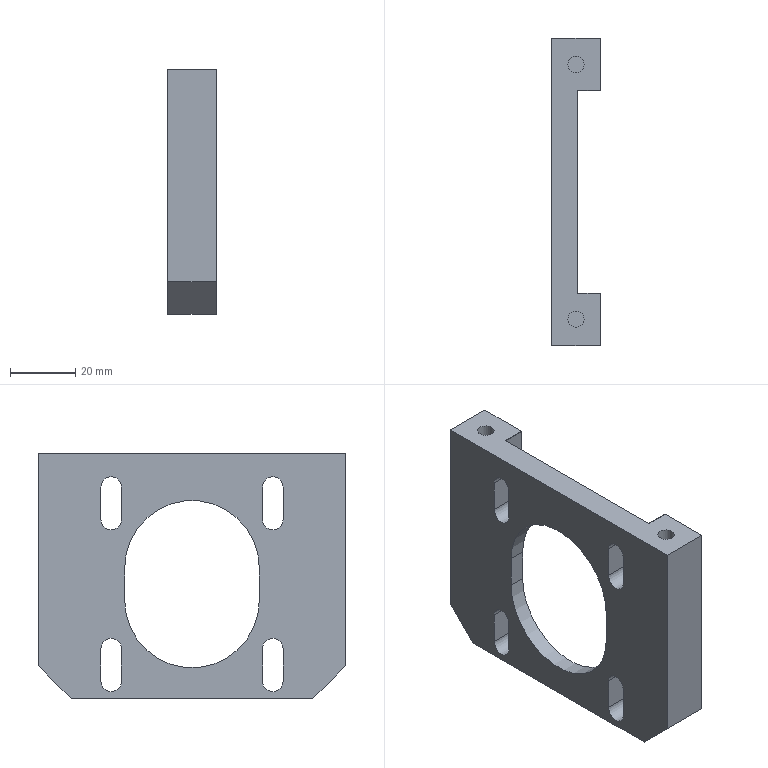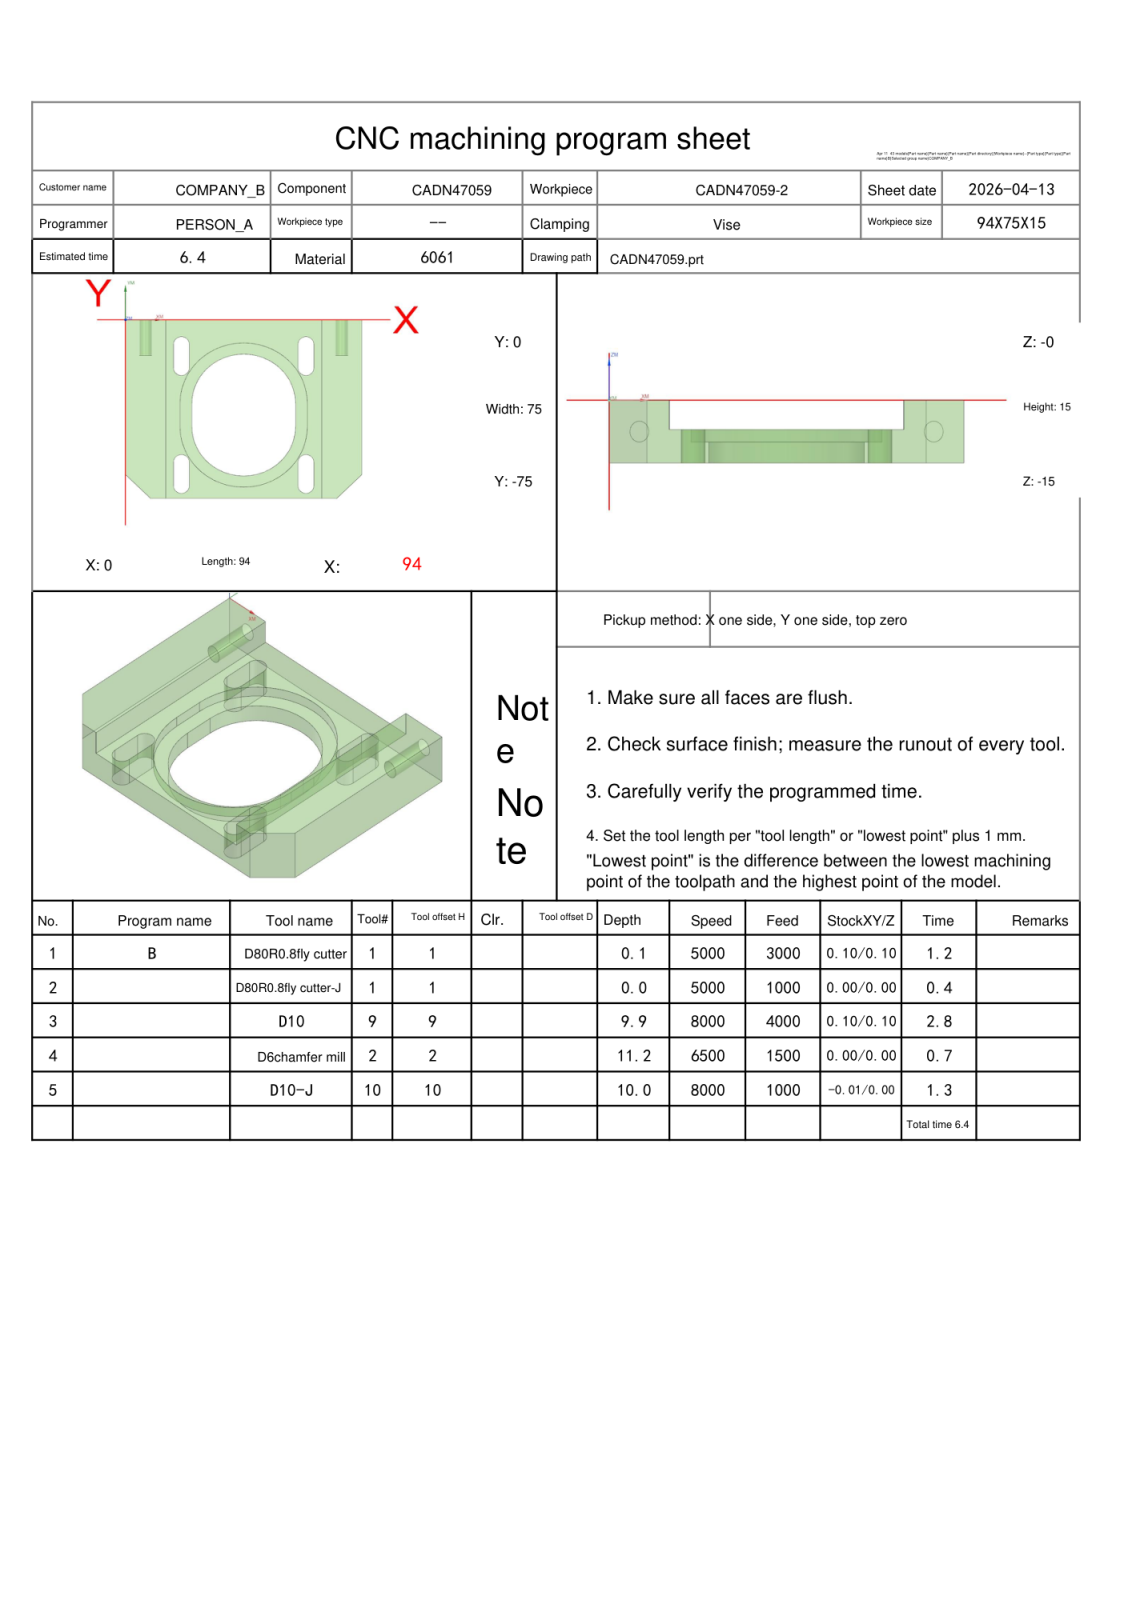NC program | NX | posted by the shop | part box 15 x 94 x 75 mm
Whole program:
%
O0001
(Machine time: 7.43 MIN)
(===Total Tool:4===)
(T1=D80R0.8 D=80.  R=0.8  D-  H01 Z=0.    )
(T9=D10     D=10.  R=0.   D-  H09 Z=-9.9  )
(T2=D6chamfer mill   D=6.   R=0.   D-  H02 Z=-11.2 )
(T10=D10-J  D=10.  R=0.   D10 H10 Z=-10.  )
G80 G90 G17 G49 G40
G91 G28 Z0
M01
N1 T01 M06
(D80R0.8  D=80. R=0.8 H=01 ce=0.10 di=0.10)
G00 G90 G54 X-52.097 Y-23.903 M03 S5000
G43 H01 Z50.
M08
Z6.011
G01 Z4.011 F3000.
X-40.097
X126.897
G02 X134.097 Y-31.103 I0.0 J-7.2
G01 Y-35.737
G02 X126.097 Y-43.737 I-8. J0.0
G01 X-40.097
X-52.097
Z6.011
G00 Y-23.903
Z5.522
G01 Z3.522
X-40.097
X126.897
G02 X134.097 Y-31.103 I0.0 J-7.2
G01 Y-35.737
G02 X126.097 Y-43.737 I-8. J0.0
G01 X-40.097
X-52.097
Z5.522
G00 Y-23.903
Z5.033
G01 Z3.033
X-40.097
X126.897
G02 X134.097 Y-31.103 I0.0 J-7.2
G01 Y-35.737
G02 X126.097 Y-43.737 I-8. J0.0
G01 X-40.097
X-52.097
Z5.033
G00 Y-23.903
Z4.544
G01 Z2.544
X-40.097
X126.897
G02 X134.097 Y-31.103 I0.0 J-7.2
G01 Y-35.737
G02 X126.097 Y-43.737 I-8. J0.0
G01 X-40.097
X-52.097
Z4.544
G00 Y-23.903
Z4.056
G01 Z2.056
X-40.097
X126.897
G02 X134.097 Y-31.103 I0.0 J-7.2
G01 Y-35.737
G02 X126.097 Y-43.737 I-8. J0.0
G01 X-40.097
X-52.097
Z4.056
G00 Y-23.903
Z3.567
G01 Z1.567
X-40.097
X126.897
G02 X134.097 Y-31.103 I0.0 J-7.2
G01 Y-35.737
G02 X126.097 Y-43.737 I-8. J0.0
G01 X-40.097
X-52.097
Z3.567
G00 Y-23.903
Z3.078
G01 Z1.078
X-40.097
X126.897
G02 X134.097 Y-31.103 I0.0 J-7.2
G01 Y-35.737
G02 X126.097 Y-43.737 I-8. J0.0
G01 X-40.097
X-52.097
Z3.078
G00 Y-23.903
Z2.589
G01 Z.589
X-40.097
X126.897
G02 X134.097 Y-31.103 I0.0 J-7.2
G01 Y-35.737
G02 X126.097 Y-43.737 I-8. J0.0
G01 X-40.097
X-52.097
Z2.589
G00 Y-23.903
Z2.1
G01 Z.1
X-40.097
X126.897
G02 X134.097 Y-31.103 I0.0 J-7.2
G01 Y-35.737
G02 X126.097 Y-43.737 I-8. J0.0
G01 X-40.097
X-52.097
Z2.1
G00 Z50.
G91 G28 Z0.0
M05
M09
G91 G28 Z0.0
M01
N2 T01 M06
(D80R0.8-J  D=80. R=0.8 H=01 ce=0.00 di=0.00)
G00 G90 G54 X-51.999 Y-24.001 M03 S5000
G43 H01 Z50.
M08
Z2.
G01 Z0.0 F1000.
X-39.999
X126.799
G02 X133.999 Y-31.201 I0.0 J-7.2
G01 Y-35.639
G02 X125.999 Y-43.639 I-8. J0.0
G01 X-39.999
X-51.999
Z2.
G00 Z50.
G91 G28 Z0.0
M05
M09
G91 G28 Z0.0
M01
N3 T09 M06
(D10  D=10. R=0. H=09 ce=0.10 di=0.10)
G00 G90 G54 X47. Y8. M03 S8000
G43 H09 Z14.8
M08
Z.925
G01 Z-.575 F4000.
Y4.9
X75.788
X72.9 Y2.012
Y-77.012
X75.788 Y-79.9
X18.212
X21.1 Y-77.012
Y2.012
X18.212 Y4.9
X43.965
G02 X44.797 Y4.455 I0.0 J-1.
G01 X49.203 Y-2.155
G03 X50.035 Y-2.6 I.832 J.555
G01 X64.402
G02 X65.4 Y-3.598 I-.002 J-1.
G01 Y-71.402
G02 X64.402 Y-72.4 I-1. J.002
G01 X29.598
G02 X28.6 Y-71.402 I.002 J1.
G01 Y-3.598
G02 X29.598 Y-2.6 I1. J-.002
G01 X43.965
G02 X44.797 Y-3.045 I0.0 J-1.
G01 X49.203 Y-9.655
G03 X50.035 Y-10.1 I.832 J.555
G01 X56.902
G02 X57.9 Y-11.098 I-.002 J-1.
G01 Y-63.902
G02 X56.902 Y-64.9 I-1. J.002
G01 X37.098
G02 X36.1 Y-63.902 I.002 J1.
G01 Y-11.098
G02 X37.098 Y-10.1 I1. J-.002
G01 X43.965
G02 X44.797 Y-10.545 I0.0 J-1.
G01 X49.29 Y-17.29
G03 X49.76 Y-17.667 I.832 J.555
G02 X50.4 Y-18.597 I-.36 J-.933
G01 Y-56.403
G02 X49.403 Y-57.4 I-1. J.003
G01 X44.597
G02 X43.6 Y-56.403 I.003 J1.
G01 Y-18.597
G02 X44.597 Y-17.6 I1. J-.003
G01 X47.
X47.5
Y-14.6
Z.925
G00 X47. Y8.
Z.35
G01 Z-1.15
Y4.9
X75.788
X72.9 Y2.012
Y-77.012
X75.788 Y-79.9
X18.212
X21.1 Y-77.012
Y2.012
X18.212 Y4.9
X43.965
G02 X44.797 Y4.455 I0.0 J-1.
G01 X49.203 Y-2.155
G03 X50.035 Y-2.6 I.832 J.555
G01 X64.402
G02 X65.4 Y-3.598 I-.002 J-1.
G01 Y-71.402
G02 X64.402 Y-72.4 I-1. J.002
G01 X29.598
G02 X28.6 Y-71.402 I.002 J1.
G01 Y-3.598
G02 X29.598 Y-2.6 I1. J-.002
G01 X43.965
G02 X44.797 Y-3.045 I0.0 J-1.
G01 X49.203 Y-9.655
G03 X50.035 Y-10.1 I.832 J.555
G01 X56.902
G02 X57.9 Y-11.098 I-.002 J-1.
G01 Y-63.902
G02 X56.902 Y-64.9 I-1. J.002
G01 X37.098
G02 X36.1 Y-63.902 I.002 J1.
G01 Y-11.098
G02 X37.098 Y-10.1 I1. J-.002
G01 X43.965
G02 X44.797 Y-10.545 I0.0 J-1.
G01 X49.29 Y-17.29
G03 X49.76 Y-17.667 I.832 J.555
G02 X50.4 Y-18.597 I-.36 J-.933
G01 Y-56.403
G02 X49.403 Y-57.4 I-1. J.003
G01 X44.597
G02 X43.6 Y-56.403 I.003 J1.
G01 Y-18.597
G02 X44.597 Y-17.6 I1. J-.003
G01 X47.
X47.5
Y-14.6
Z.35
G00 X47. Y8.
Z-.225
G01 Z-1.725
Y4.9
X75.788
X72.9 Y2.012
Y-77.012
X75.788 Y-79.9
X18.212
X21.1 Y-77.012
Y2.012
X18.212 Y4.9
X43.965
G02 X44.797 Y4.455 I0.0 J-1.
G01 X49.203 Y-2.155
G03 X50.035 Y-2.6 I.832 J.555
G01 X64.402
G02 X65.4 Y-3.598 I-.002 J-1.
G01 Y-71.402
G02 X64.402 Y-72.4 I-1. J.002
G01 X29.598
G02 X28.6 Y-71.402 I.002 J1.
G01 Y-3.598
G02 X29.598 Y-2.6 I1. J-.002
G01 X43.965
G02 X44.797 Y-3.045 I0.0 J-1.
G01 X49.203 Y-9.655
G03 X50.035 Y-10.1 I.832 J.555
G01 X56.902
G02 X57.9 Y-11.098 I-.002 J-1.
G01 Y-63.902
G02 X56.902 Y-64.9 I-1. J.002
G01 X37.098
G02 X36.1 Y-63.902 I.002 J1.
G01 Y-11.098
G02 X37.098 Y-10.1 I1. J-.002
G01 X43.965
G02 X44.797 Y-10.545 I0.0 J-1.
G01 X49.29 Y-17.29
G03 X49.76 Y-17.667 I.832 J.555
G02 X50.4 Y-18.597 I-.36 J-.933
G01 Y-56.403
G02 X49.403 Y-57.4 I-1. J.003
G01 X44.597
G02 X43.6 Y-56.403 I.003 J1.
G01 Y-18.597
G02 X44.597 Y-17.6 I1. J-.003
G01 X47.
X47.5
Y-14.6
Z-.225
G00 X47. Y8.
Z-.8
G01 Z-2.3
Y4.9
X75.788
X72.9 Y2.012
Y-77.012
X75.788 Y-79.9
X18.212
X21.1 Y-77.012
Y2.012
X18.212 Y4.9
X43.965
G02 X44.797 Y4.455 I0.0 J-1.
G01 X49.203 Y-2.155
G03 X50.035 Y-2.6 I.832 J.555
G01 X64.402
G02 X65.4 Y-3.598 I-.002 J-1.
G01 Y-71.402
G02 X64.402 Y-72.4 I-1. J.002
G01 X29.598
G02 X28.6 Y-71.402 I.002 J1.
G01 Y-3.598
G02 X29.598 Y-2.6 I1. J-.002
G01 X43.965
G02 X44.797 Y-3.045 I0.0 J-1.
G01 X49.203 Y-9.655
G03 X50.035 Y-10.1 I.832 J.555
G01 X56.902
G02 X57.9 Y-11.098 I-.002 J-1.
G01 Y-63.902
G02 X56.902 Y-64.9 I-1. J.002
G01 X37.098
G02 X36.1 Y-63.902 I.002 J1.
G01 Y-11.098
G02 X37.098 Y-10.1 I1. J-.002
G01 X43.965
G02 X44.797 Y-10.545 I0.0 J-1.
G01 X49.29 Y-17.29
G03 X49.76 Y-17.667 I.832 J.555
G02 X50.4 Y-18.597 I-.36 J-.933
G01 Y-56.403
G02 X49.403 Y-57.4 I-1. J.003
G01 X44.597
G02 X43.6 Y-56.403 I.003 J1.
G01 Y-18.597
G02 X44.597 Y-17.6 I1. J-.003
G01 X47.
X47.5
Y-14.6
Z-.8
G00 X47. Y8.
Z-1.375
G01 Z-2.875
Y4.9
X75.788
X72.9 Y2.012
Y-77.012
X75.788 Y-79.9
X18.212
X21.1 Y-77.012
Y2.012
X18.212 Y4.9
X43.965
G02 X44.797 Y4.455 I0.0 J-1.
G01 X49.203 Y-2.155
G03 X50.035 Y-2.6 I.832 J.555
G01 X64.402
G02 X65.4 Y-3.598 I-.002 J-1.
G01 Y-71.402
G02 X64.402 Y-72.4 I-1. J.002
G01 X29.598
G02 X28.6 Y-71.402 I.002 J1.
G01 Y-3.598
G02 X29.598 Y-2.6 I1. J-.002
G01 X43.965
G02 X44.797 Y-3.045 I0.0 J-1.
G01 X49.203 Y-9.655
G03 X50.035 Y-10.1 I.832 J.555
G01 X56.902
G02 X57.9 Y-11.098 I-.002 J-1.
G01 Y-63.902
G02 X56.902 Y-64.9 I-1. J.002
G01 X37.098
G02 X36.1 Y-63.902 I.002 J1.
G01 Y-11.098
G02 X37.098 Y-10.1 I1. J-.002
G01 X43.965
G02 X44.797 Y-10.545 I0.0 J-1.
G01 X49.29 Y-17.29
G03 X49.76 Y-17.667 I.832 J.555
G02 X50.4 Y-18.597 I-.36 J-.933
G01 Y-56.403
G02 X49.403 Y-57.4 I-1. J.003
G01 X44.597
G02 X43.6 Y-56.403 I.003 J1.
G01 Y-18.597
G02 X44.597 Y-17.6 I1. J-.003
G01 X47.
X47.5
Y-14.6
Z-1.375
G00 X47. Y8.
Z-1.95
G01 Z-3.45
Y4.9
X75.788
X72.9 Y2.012
Y-77.012
X75.788 Y-79.9
X18.212
X21.1 Y-77.012
Y2.012
X18.212 Y4.9
X43.965
G02 X44.797 Y4.455 I0.0 J-1.
G01 X49.203 Y-2.155
G03 X50.035 Y-2.6 I.832 J.555
G01 X64.402
G02 X65.4 Y-3.598 I-.002 J-1.
G01 Y-71.402
G02 X64.402 Y-72.4 I-1. J.002
G01 X29.598
G02 X28.6 Y-71.402 I.002 J1.
G01 Y-3.598
G02 X29.598 Y-2.6 I1. J-.002
G01 X43.965
G02 X44.797 Y-3.045 I0.0 J-1.
G01 X49.203 Y-9.655
G03 X50.035 Y-10.1 I.832 J.555
G01 X56.902
G02 X57.9 Y-11.098 I-.002 J-1.
G01 Y-63.902
G02 X56.902 Y-64.9 I-1. J.002
G01 X37.098
G02 X36.1 Y-63.902 I.002 J1.
G01 Y-11.098
G02 X37.098 Y-10.1 I1. J-.002
G01 X43.965
G02 X44.797 Y-10.545 I0.0 J-1.
G01 X49.29 Y-17.29
G03 X49.76 Y-17.667 I.832 J.555
G02 X50.4 Y-18.597 I-.36 J-.933
G01 Y-56.403
G02 X49.403 Y-57.4 I-1. J.003
G01 X44.597
G02 X43.6 Y-56.403 I.003 J1.
G01 Y-18.597
G02 X44.597 Y-17.6 I1. J-.003
G01 X47.
X47.5
Y-14.6
Z-1.95
G00 X47. Y8.
Z-2.525
G01 Z-4.025
Y4.9
X75.788
X72.9 Y2.012
Y-77.012
X75.788 Y-79.9
X18.212
X21.1 Y-77.012
Y2.012
X18.212 Y4.9
X43.965
G02 X44.797 Y4.455 I0.0 J-1.
G01 X49.203 Y-2.155
G03 X50.035 Y-2.6 I.832 J.555
G01 X64.402
G02 X65.4 Y-3.598 I-.002 J-1.
G01 Y-71.402
G02 X64.402 Y-72.4 I-1. J.002
G01 X29.598
G02 X28.6 Y-71.402 I.002 J1.
G01 Y-3.598
G02 X29.598 Y-2.6 I1. J-.002
G01 X43.965
G02 X44.797 Y-3.045 I0.0 J-1.
G01 X49.203 Y-9.655
G03 X50.035 Y-10.1 I.832 J.555
G01 X56.902
G02 X57.9 Y-11.098 I-.002 J-1.
G01 Y-63.902
G02 X56.902 Y-64.9 I-1. J.002
G01 X37.098
G02 X36.1 Y-63.902 I.002 J1.
G01 Y-11.098
G02 X37.098 Y-10.1 I1. J-.002
G01 X43.965
G02 X44.797 Y-10.545 I0.0 J-1.
G01 X49.29 Y-17.29
G03 X49.76 Y-17.667 I.832 J.555
G02 X50.4 Y-18.597 I-.36 J-.933
G01 Y-56.403
G02 X49.403 Y-57.4 I-1. J.003
G01 X44.597
G02 X43.6 Y-56.403 I.003 J1.
G01 Y-18.597
G02 X44.597 Y-17.6 I1. J-.003
G01 X47.
X47.5
Y-14.6
Z-2.525
G00 X47. Y8.
Z-3.1
G01 Z-4.6
Y4.9
X75.788
X72.9 Y2.012
Y-77.012
X75.788 Y-79.9
X18.212
X21.1 Y-77.012
Y2.012
X18.212 Y4.9
X43.965
G02 X44.797 Y4.455 I0.0 J-1.
G01 X49.203 Y-2.155
G03 X50.035 Y-2.6 I.832 J.555
G01 X64.402
G02 X65.4 Y-3.598 I-.002 J-1.
G01 Y-71.402
G02 X64.402 Y-72.4 I-1. J.002
G01 X29.598
G02 X28.6 Y-71.402 I.002 J1.
G01 Y-3.598
G02 X29.598 Y-2.6 I1. J-.002
G01 X43.965
G02 X44.797 Y-3.045 I0.0 J-1.
G01 X49.203 Y-9.655
G03 X50.035 Y-10.1 I.832 J.555
G01 X56.902
G02 X57.9 Y-11.098 I-.002 J-1.
G01 Y-63.902
G02 X56.902 Y-64.9 I-1. J.002
G01 X37.098
G02 X36.1 Y-63.902 I.002 J1.
G01 Y-11.098
G02 X37.098 Y-10.1 I1. J-.002
G01 X43.965
G02 X44.797 Y-10.545 I0.0 J-1.
G01 X49.29 Y-17.29
G03 X49.76 Y-17.667 I.832 J.555
G02 X50.4 Y-18.597 I-.36 J-.933
G01 Y-56.403
G02 X49.403 Y-57.4 I-1. J.003
G01 X44.597
G02 X43.6 Y-56.403 I.003 J1.
G01 Y-18.597
G02 X44.597 Y-17.6 I1. J-.003
G01 X47.
X47.5
Y-14.6
Z-3.1
G00 X47. Y8.
Z-3.675
G01 Z-5.175
Y4.9
X75.788
X72.9 Y2.012
Y-77.012
X75.788 Y-79.9
X18.212
X21.1 Y-77.012
Y2.012
X18.212 Y4.9
X43.965
G02 X44.797 Y4.455 I0.0 J-1.
G01 X49.203 Y-2.155
G03 X50.035 Y-2.6 I.832 J.555
G01 X64.402
G02 X65.4 Y-3.598 I-.002 J-1.
G01 Y-71.402
G02 X64.402 Y-72.4 I-1. J.002
G01 X29.598
G02 X28.6 Y-71.402 I.002 J1.
G01 Y-3.598
G02 X29.598 Y-2.6 I1. J-.002
G01 X43.965
G02 X44.797 Y-3.045 I0.0 J-1.
G01 X49.203 Y-9.655
G03 X50.035 Y-10.1 I.832 J.555
G01 X56.902
G02 X57.9 Y-11.098 I-.002 J-1.
G01 Y-63.902
G02 X56.902 Y-64.9 I-1. J.002
G01 X37.098
G02 X36.1 Y-63.902 I.002 J1.
G01 Y-11.098
G02 X37.098 Y-10.1 I1. J-.002
G01 X43.965
G02 X44.797 Y-10.545 I0.0 J-1.
G01 X49.29 Y-17.29
G03 X49.76 Y-17.667 I.832 J.555
G02 X50.4 Y-18.597 I-.36 J-.933
G01 Y-56.403
G02 X49.403 Y-57.4 I-1. J.003
G01 X44.597
G02 X43.6 Y-56.403 I.003 J1.
G01 Y-18.597
G02 X44.597 Y-17.6 I1. J-.003
G01 X47.
X47.5
Y-14.6
Z-3.675
G00 X47. Y8.
Z-4.25
G01 Z-5.75
Y4.9
X75.788
X72.9 Y2.012
Y-77.012
X75.788 Y-79.9
X18.212
X21.1 Y-77.012
Y2.012
X18.212 Y4.9
X43.965
G02 X44.797 Y4.455 I0.0 J-1.
G01 X49.203 Y-2.155
G03 X50.035 Y-2.6 I.832 J.555
G01 X64.402
G02 X65.4 Y-3.598 I-.002 J-1.
G01 Y-71.402
G02 X64.402 Y-72.4 I-1. J.002
G01 X29.598
G02 X28.6 Y-71.402 I.002 J1.
G01 Y-3.598
G02 X29.598 Y-2.6 I1. J-.002
G01 X43.965
G02 X44.797 Y-3.045 I0.0 J-1.
G01 X49.203 Y-9.655
G03 X50.035 Y-10.1 I.832 J.555
G01 X56.902
G02 X57.9 Y-11.098 I-.002 J-1.
G01 Y-63.902
G02 X56.902 Y-64.9 I-1. J.002
G01 X37.098
G02 X36.1 Y-63.902 I.002 J1.
G01 Y-11.098
G02 X37.098 Y-10.1 I1. J-.002
G01 X43.965
G02 X44.797 Y-10.545 I0.0 J-1.
G01 X49.29 Y-17.29
G03 X49.76 Y-17.667 I.832 J.555
G02 X50.4 Y-18.597 I-.36 J-.933
G01 Y-56.403
G02 X49.403 Y-57.4 I-1. J.003
G01 X44.597
G02 X43.6 Y-56.403 I.003 J1.
G01 Y-18.597
G02 X44.597 Y-17.6 I1. J-.003
G01 X47.
X47.5
Y-14.6
Z-4.25
G00 X47. Y8.
Z-4.825
G01 Z-6.325
Y4.9
X75.788
X72.9 Y2.012
Y-77.012
X75.788 Y-79.9
X18.212
X21.1 Y-77.012
Y2.012
X18.212 Y4.9
X43.965
G02 X44.797 Y4.455 I0.0 J-1.
G01 X49.203 Y-2.155
G03 X50.035 Y-2.6 I.832 J.555
G01 X64.402
G02 X65.4 Y-3.598 I-.002 J-1.
G01 Y-71.402
G02 X64.402 Y-72.4 I-1. J.002
G01 X29.598
G02 X28.6 Y-71.402 I.002 J1.
G01 Y-3.598
G02 X29.598 Y-2.6 I1. J-.002
G01 X43.965
G02 X44.797 Y-3.045 I0.0 J-1.
G01 X49.203 Y-9.655
G03 X50.035 Y-10.1 I.832 J.555
G01 X56.902
G02 X57.9 Y-11.098 I-.002 J-1.
G01 Y-63.902
G02 X56.902 Y-64.9 I-1. J.002
G01 X37.098
G02 X36.1 Y-63.902 I.002 J1.
G01 Y-11.098
G02 X37.098 Y-10.1 I1. J-.002
G01 X43.965
G02 X44.797 Y-10.545 I0.0 J-1.
G01 X49.29 Y-17.29
G03 X49.76 Y-17.667 I.832 J.555
G02 X50.4 Y-18.597 I-.36 J-.933
G01 Y-56.403
G02 X49.403 Y-57.4 I-1. J.003
G01 X44.597
G02 X43.6 Y-56.403 I.003 J1.
G01 Y-18.597
G02 X44.597 Y-17.6 I1. J-.003
G01 X47.
X47.5
Y-14.6
Z-4.825
G00 X47. Y8.
Z-5.4
G01 Z-6.9
Y4.9
X75.788
X72.9 Y2.012
Y-77.012
X75.788 Y-79.9
X18.212
X21.1 Y-77.012
Y2.012
X18.212 Y4.9
X43.965
G02 X44.797 Y4.455 I0.0 J-1.
G01 X49.203 Y-2.155
G03 X50.035 Y-2.6 I.832 J.555
G01 X64.402
G02 X65.4 Y-3.598 I-.002 J-1.
G01 Y-71.402
G02 X64.402 Y-72.4 I-1. J.002
G01 X29.598
G02 X28.6 Y-71.402 I.002 J1.
G01 Y-3.598
G02 X29.598 Y-2.6 I1. J-.002
G01 X43.965
G02 X44.797 Y-3.045 I0.0 J-1.
G01 X49.203 Y-9.655
G03 X50.035 Y-10.1 I.832 J.555
G01 X56.902
G02 X57.9 Y-11.098 I-.002 J-1.
G01 Y-63.902
G02 X56.902 Y-64.9 I-1. J.002
G01 X37.098
G02 X36.1 Y-63.902 I.002 J1.
G01 Y-11.098
G02 X37.098 Y-10.1 I1. J-.002
G01 X43.965
G02 X44.797 Y-10.545 I0.0 J-1.
G01 X49.29 Y-17.29
G03 X49.76 Y-17.667 I.832 J.555
G02 X50.4 Y-18.597 I-.36 J-.933
G01 Y-56.403
G02 X49.403 Y-57.4 I-1. J.003
G01 X44.597
G02 X43.6 Y-56.403 I.003 J1.
G01 Y-18.597
G02 X44.597 Y-17.6 I1. J-.003
G01 X47.
X47.5
Y-14.6
Z-5.4
G00 Z14.8
G00 G90 X35.144 Y-18.629 M03 S8000
Z50.
Z-6.
G01 X34.932 Y-18.764 Z-6.013 F2000.
X32.695 Y-20.695 Z-6.168
X30.764 Y-22.932 Z-6.323
X29.179 Y-25.425 Z-6.478
X27.975 Y-28.123 Z-6.633
X27.176 Y-30.968 Z-6.787
X26.8 Y-33.899 Z-6.942
Y-35. Z-7.
Y-45. Z-7.039
G03 X47. Y-65.2 Z-7.165 I20.2 J0.0
X67.2 Y-45. Z-7.29 I0.0 J20.2
G01 Y-35. Z-7.329
G03 X47. Y-14.8 Z-7.455 I-20.2 J0.0
X26.8 Y-35. Z-7.58 I0.0 J-20.2
G01 Y-45. Z-7.619
G03 X47. Y-65.2 Z-7.745 I20.2 J0.0
X67.2 Y-45. Z-7.87 I0.0 J20.2
G01 Y-35. Z-7.909
G03 X47. Y-14.8 Z-8.035 I-20.2 J0.0
X26.8 Y-35. Z-8.16 I0.0 J-20.2
G01 Y-45. Z-8.199
G03 X47. Y-65.2 Z-8.325 I20.2 J0.0
X67.2 Y-45. Z-8.45 I0.0 J20.2
G01 Y-35. Z-8.489
G03 X47. Y-14.8 Z-8.615 I-20.2 J0.0
X26.8 Y-35. Z-8.74 I0.0 J-20.2
G01 Y-45. Z-8.779
G03 X47. Y-65.2 Z-8.905 I20.2 J0.0
X67.2 Y-45. Z-9.03 I0.0 J20.2
G01 Y-35. Z-9.069
G03 X47. Y-14.8 Z-9.195 I-20.2 J0.0
X26.8 Y-35. Z-9.32 I0.0 J-20.2
G01 Y-45. Z-9.359
G03 X47. Y-65.2 Z-9.485 I20.2 J0.0
X67.2 Y-45. Z-9.61 I0.0 J20.2
G01 Y-35. Z-9.649
G03 X47. Y-14.8 Z-9.775 I-20.2 J0.0
X26.8 Y-35. Z-9.9 I0.0 J-20.2
G01 Y-45.
G03 X47. Y-65.2 I20.2 J0.0
X67.2 Y-45. I0.0 J20.2
G01 Y-35.
G03 X47. Y-14.8 I-20.2 J0.0
X26.8 Y-35. I0.0 J-20.2
G01 Y-35.4
Z-8.9
G00 Z50.
G91 G28 Z0.0
M05
M09
G91 G28 Z0.0
M01
N4 T02 M06
(D6chamfer mill  D=6. R=0. H=02 ce=0.00 di=0.00)
G00 G90 G54 X76.773 Y-37.886 M03 S6500
G43 H02 Z50.
M08
Z.172
G01 Z-1.199 F1500.
G03 X76.973 Y-37.6 I-1.532 J1.286
G01 X77.003 Y-37.554
X77. Y-37.5
Y-.1
X77.034 Y.159
X77.134 Y.4
X77.293 Y.607
X77.393 Y.707
X77.6 Y.866
X77.841 Y.966
X78.1 Y1.
X94.
G02 X95. Y0.0 I0.0 J-1.
G01 Y-65.
X94.966 Y-65.259
X94.866 Y-65.5
X94.707 Y-65.707
X84.707 Y-75.707
X84.5 Y-75.866
X84.259 Y-75.966
X84. Y-76.
X78.1
X77.841 Y-75.966
X77.6 Y-75.866
X77.393 Y-75.707
X77.293 Y-75.607
X77.134 Y-75.4
X77.034 Y-75.159
X77. Y-74.9
Y-37.5
X77.003 Y-37.446
X76.973 Y-37.4
G03 X76.773 Y-37.114 I-1.732 J-1.
G01 Z.172
G00 Z10.
X17.227
Z.172
G01 Z-1.199
G03 X17.027 Y-37.4 I1.532 J-1.286
G01 X16.997 Y-37.446
X17. Y-37.5
Y-74.9
X16.966 Y-75.159
X16.866 Y-75.4
X16.707 Y-75.607
X16.607 Y-75.707
X16.4 Y-75.866
X16.159 Y-75.966
X15.9 Y-76.
X10.
X9.741 Y-75.966
X9.5 Y-75.866
X9.293 Y-75.707
X-.707 Y-65.707
X-.866 Y-65.5
X-.966 Y-65.259
X-1. Y-65.
Y0.0
G02 X0.0 Y1. I1. J0.0
G01 X15.9
X16.159 Y.966
X16.4 Y.866
X16.607 Y.707
X16.707 Y.607
X16.866 Y.4
X16.966 Y.159
X17. Y-.1
Y-37.5
X16.997 Y-37.554
X17.027 Y-37.6
G03 X17.227 Y-37.886 I1.732 J1.
G01 Z.172
G00 Z10.
X75.027 Y-76.068
Z-1.796
G01 Z-8.199
X74.941 Y-76.008
X74.911 Y-76.
X19.089
X19.059 Y-76.008
X18.973 Y-76.068
Z-1.796
G00 Z10.
Y1.068
Z-1.796
G01 Z-8.199
X19.059 Y1.008
X19.089 Y1.
X74.911
X74.941 Y1.008
X75.027 Y1.068
Z-1.796
G00 Z10.
X24.175 Y-65.134
Z-6.828
G01 Z-8.199
G03 X24.374 Y-64.849 I-1.532 J1.286
G01 X24.404 Y-64.803
X24.401 Y-64.749
Y-59.749
G03 X22.251 Y-57.599 I-2.15 J0.0
X20.101 Y-59.749 I0.0 J-2.15
G01 Y-69.749
G03 X22.251 Y-71.899 I2.15 J0.0
X24.401 Y-69.749 I0.0 J2.15
G01 Y-64.749
X24.404 Y-64.694
X24.374 Y-64.649
G03 X24.175 Y-64.363 I-1.732 J-1.
G01 Z-6.828
G00 Z10.
Y-15.637
Z-6.828
G01 Z-8.199
G03 X24.374 Y-15.351 I-1.532 J1.286
G01 X24.404 Y-15.306
X24.401 Y-15.251
Y-10.251
G03 X22.251 Y-8.101 I-2.15 J0.0
X20.101 Y-10.251 I0.0 J-2.15
G01 Y-20.251
G03 X22.251 Y-22.401 I2.15 J0.0
X24.401 Y-20.251 I0.0 J2.15
G01 Y-15.251
X24.404 Y-15.197
X24.374 Y-15.151
G03 X24.175 Y-14.866 I-1.732 J-1.
G01 Z-6.828
G00 Z10.
X22.927 Y-39.614
Z-6.828
G01 Z-8.199
G03 X22.727 Y-39.9 I1.532 J-1.286
G01 X22.697 Y-39.946
X22.7 Y-40.
Y-45.
G03 X47. Y-69.3 I24.3 J0.0
X71.3 Y-45. I0.0 J24.3
G01 Y-35.
G03 X47. Y-10.7 I-24.3 J0.0
X22.7 Y-35. I0.0 J-24.3
G01 Y-40.
X22.697 Y-40.054
X22.727 Y-40.1
G03 X22.927 Y-40.386 I1.732 J1.
G01 Z-6.828
G00 Z10.
X69.825 Y-14.866
Z-6.828
G01 Z-8.199
G03 X69.626 Y-15.151 I1.532 J-1.286
G01 X69.596 Y-15.197
X69.599 Y-15.251
Y-20.251
G03 X71.749 Y-22.401 I2.15 J0.0
X73.899 Y-20.251 I0.0 J2.15
G01 Y-10.251
G03 X71.749 Y-8.101 I-2.15 J0.0
X69.599 Y-10.251 I0.0 J-2.15
G01 Y-15.251
X69.596 Y-15.306
X69.626 Y-15.351
G03 X69.825 Y-15.637 I1.732 J1.
G01 Z-6.828
G00 Z10.
Y-64.363
Z-6.828
G01 Z-8.199
G03 X69.626 Y-64.649 I1.532 J-1.286
G01 X69.596 Y-64.694
X69.599 Y-64.749
Y-69.749
G03 X71.749 Y-71.899 I2.15 J0.0
X73.899 Y-69.749 I0.0 J2.15
G01 Y-59.749
G03 X71.749 Y-57.599 I-2.15 J0.0
X69.599 Y-59.749 I0.0 J-2.15
G01 Y-64.749
X69.596 Y-64.803
X69.626 Y-64.849
G03 X69.825 Y-65.134 I1.732 J1.
G01 Z-6.828
G00 Z10.
X66.373 Y-40.386
Z-9.828
G01 Z-11.199
G03 X66.573 Y-40.1 I-1.532 J1.286
G01 X66.603 Y-40.054
X66.6 Y-40.
Y-35.
G03 X47. Y-15.4 I-19.6 J0.0
X27.4 Y-35. I0.0 J-19.6
G01 Y-45.
G03 X47. Y-64.6 I19.6 J0.0
X66.6 Y-45. I0.0 J19.6
G01 Y-40.
X66.603 Y-39.946
X66.573 Y-39.9
G03 X66.373 Y-39.614 I-1.732 J-1.
G01 Z-9.828
G00 Z50.
G91 G28 Z0.0
M05
M09
G91 G28 Z0.0
M01
N5 T10 M06
(D10-J  D=10. R=0. H=10 ce=0.40 di=0.00)
G00 G90 G54 X49. Y-82. M03 S8000
G43 H10 Z14.8
M08
Z-5.5
G01 Z-7. F1000.
Y-78.
G03 X47. Y-76. I-2. J0.0
G01 X22.397
G02 X21.4 Y-75.003 I.003 J1.
G01 Y.003
G02 X22.397 Y1. I1. J-.003
G01 X71.603
G02 X72.6 Y.003 I-.003 J-1.
G01 Y-75.003
G02 X71.603 Y-76. I-1. J.003
G01 X44.914
G02 X44.207 Y-75.707 I0.0 J1.
G01 X39.793 Y-71.293
G03 X39.086 Y-71. I-.707 J-.707
G01 X27.397
G02 X26.4 Y-70.003 I.003 J1.
G01 Y-4.997
G02 X27.397 Y-4. I1. J-.003
G01 X66.603
G02 X67.6 Y-4.997 I-.003 J-1.
G01 Y-70.003
G02 X66.603 Y-71. I-1. J.003
G01 X44.914
G02 X44.207 Y-70.707 I0.0 J1.
G01 X39.793 Y-66.293
G03 X39.086 Y-66. I-.707 J-.707
G01 X32.397
G02 X31.4 Y-65.003 I.003 J1.
G01 Y-9.997
G02 X32.397 Y-9. I1. J-.003
G01 X61.603
G02 X62.6 Y-9.997 I-.003 J-1.
G01 Y-65.003
G02 X61.603 Y-66. I-1. J.003
G01 X44.914
G02 X44.207 Y-65.707 I0.0 J1.
G01 X39.793 Y-61.293
G03 X39.086 Y-61. I-.707 J-.707
G01 X37.397
G02 X36.4 Y-60.003 I.003 J1.
G01 Y-14.997
G02 X37.397 Y-14. I1. J-.003
G01 X56.603
G02 X57.6 Y-14.997 I-.003 J-1.
G01 Y-60.003
G02 X56.603 Y-61. I-1. J.003
G01 X45.157
G02 X44.239 Y-60.397 I0.0 J1.
G01 X42.524 Y-56.438
G03 X42.004 Y-55.918 I-.917 J-.398
G02 X41.4 Y-55.003 I.396 J.918
G01 Y-19.997
G02 X42.397 Y-19. I1. J-.003
G01 X51.603
G02 X52.6 Y-19.997 I-.003 J-1.
G01 Y-55.003
G02 X51.603 Y-56. I-1. J.003
G01 X45.816
G02 X45.016 Y-55.2 I0.0 J.8
G01 X45.032 Y-55.038
X46.379 Y-48.525
G03 X46.4 Y-48.324 I-.979 J.202
G01 Y-24.597
G02 X47. Y-24. I.6 J-.003
G01 X47.003
G02 X47.6 Y-24.597 I-.003 J-.6
G01 Y-50.403
G02 X47. Y-51. I-.6 J.003
G01 X46.997
G02 X46.616 Y-50.861 I.003 J.6
X46.4 Y-50.403 I.384 J.461
G01 Y-49.926
G03 X44.4 Y-47.926 I-2. J0.0
G01 Z-5.5
G00 Z14.8
G00 G90 X76.496 Y-82.177 M03 S8000
Z14.8
Z-6.
G01 Z-7. F1000.
G41 D10
X76.553 Y-81.985
G03 X76.636 Y-81.414 I-1.917 J.571
X76.05 Y-80. I-2. J0.0
G01 X73.015 Y-76.965
Y1.965
X76.05 Y5.
G03 X76.636 Y6.414 I-1.414 J1.414
X76.553 Y6.985 I-2. J0.0
G01 G40 X76.496 Y7.177
Z-6.
G00 X17.504
G01 Z-7.
G41 D10
X17.447 Y6.985
G03 X17.364 Y6.414 I1.917 J-.571
X17.95 Y5. I2. J0.0
G01 X20.985 Y1.965
Y-76.965
X17.95 Y-80.
G03 X17.364 Y-81.414 I1.414 J-1.414
X17.447 Y-81.985 I2. J0.0
G01 G40 X17.504 Y-82.177
Z-6.
G00 Z14.8
G00 G90 X35.048 Y-33. M03 S8000
Z14.8
Z-9.
G01 Z-10. F1000.
G41 D10
X28.685
G03 X26.685 Y-35. I0.0 J-2.
G01 Y-45.
G03 X47. Y-65.315 I20.315 J0.0
X67.315 Y-45. I0.0 J20.315
G01 Y-35.
G03 X47. Y-14.685 I-20.315 J0.0
X26.685 Y-35. I0.0 J-20.315
G01 Y-35.4
G03 X28.685 Y-37.4 I2. J0.0
G01 X34.685
G40 X34.885
Z-9.
G00 Z14.8
M05
M09
G91 G28 Z0.0
G91 G28 Y0.0
M30
%